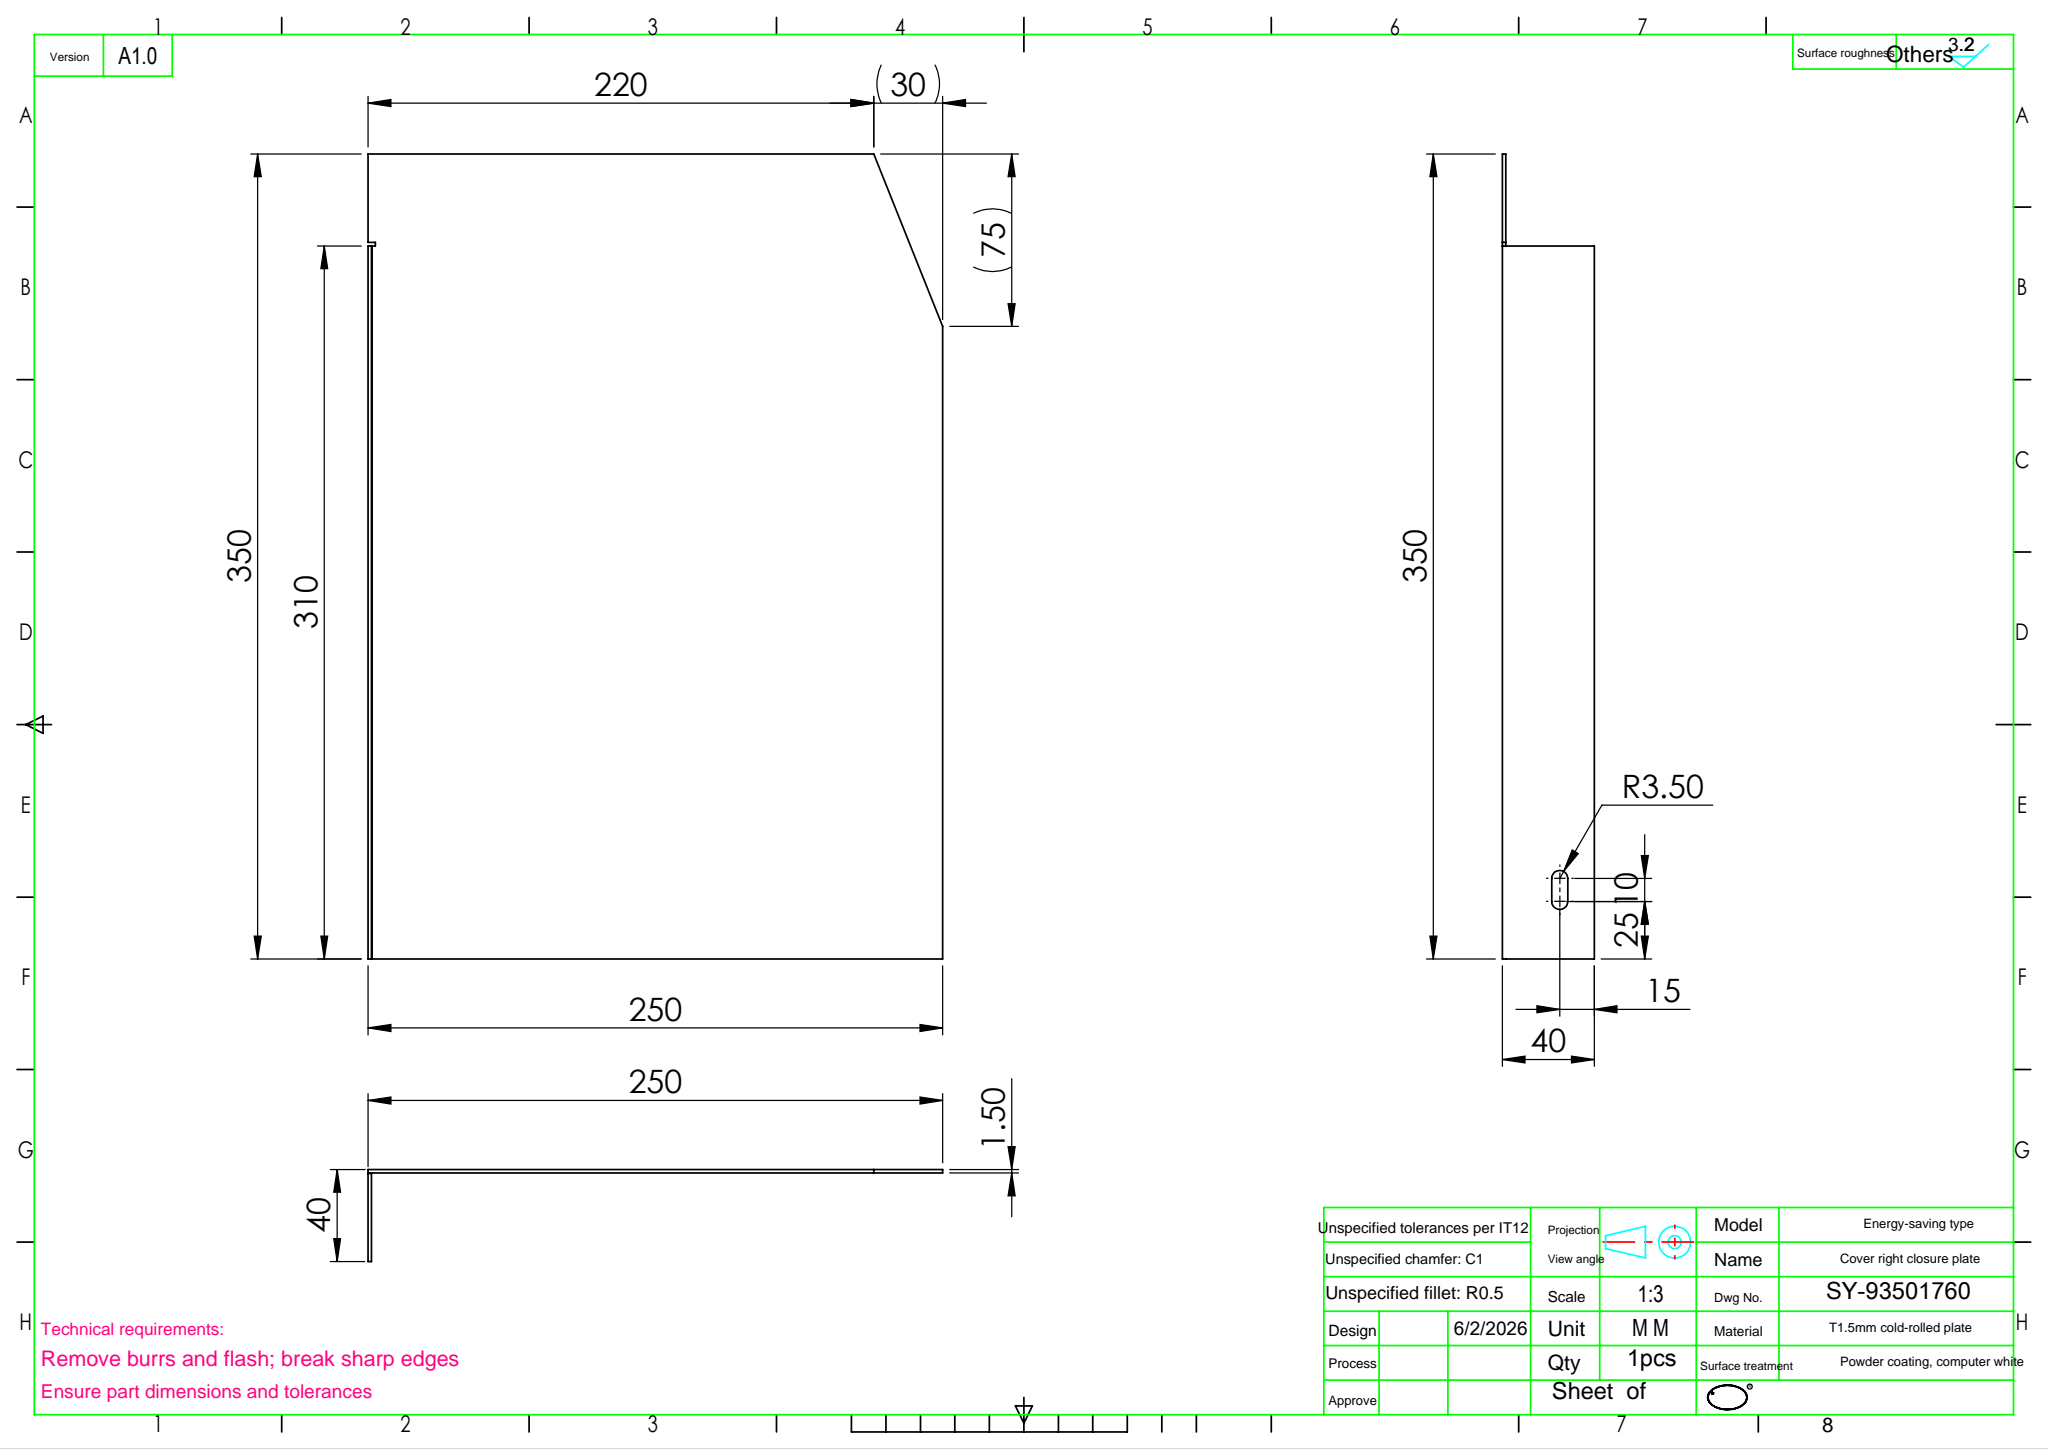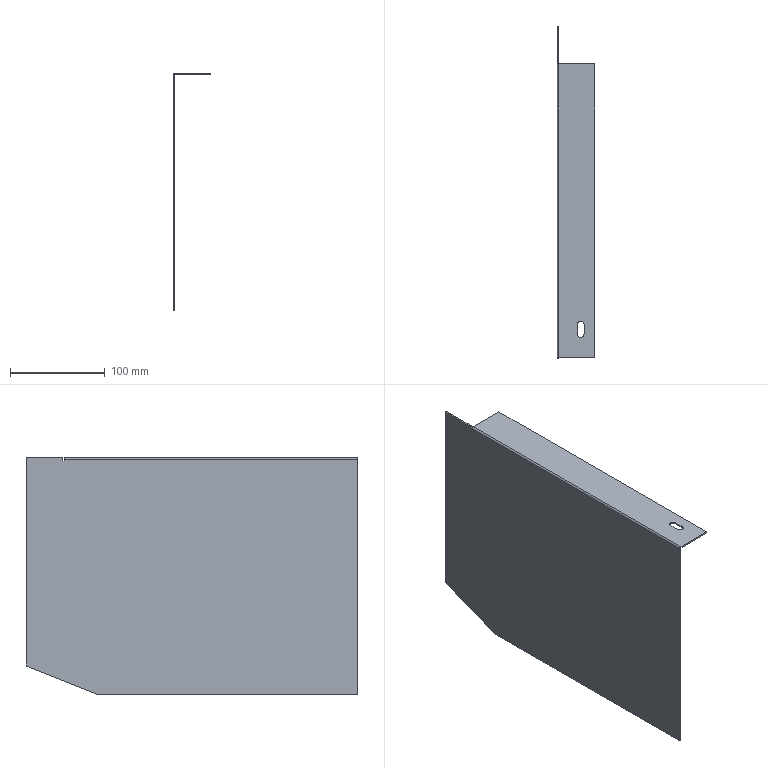Part | SolidWorks | features EdgeFlange 1, FlatPattern 1, ICE 1, SMBaseFlange 1, SheetMetal 1 | 1 solid | 24 faces | box 40 x 350 x 250 mm | volume 147105 mm3 | plane 19 | cylinder 5 | commonest cylinder face diameters 7 x3 0.4 x1 3.4 x1
STEP:
#1=CARTESIAN_POINT('',(23.5,38.5,0.));
#2=VERTEX_POINT('',#1);
#3=CARTESIAN_POINT('',(27.,35.,0.));
#4=VERTEX_POINT('',#3);
#5=CARTESIAN_POINT('',(23.5,35.,0.));
#6=DIRECTION('',(0.,0.,-1.));
#7=DIRECTION('',(-1.,0.,0.));
#8=AXIS2_PLACEMENT_3D('',#5,#6,#7);
#9=CIRCLE('',#8,3.5);
#10=EDGE_CURVE('',#2,#4,#9,.T.);
#11=ORIENTED_EDGE('',*,*,#10,.F.);
#12=CARTESIAN_POINT('',(23.5,38.5,-1.5));
#13=VERTEX_POINT('',#12);
#14=CARTESIAN_POINT('',(23.5,38.5,8.5));
#15=DIRECTION('',(0.,0.,-1.));
#16=VECTOR('',#15,1000.);
#17=LINE('',#14,#16);
#18=EDGE_CURVE('',#2,#13,#17,.T.);
#19=ORIENTED_EDGE('',*,*,#18,.T.);
#20=CARTESIAN_POINT('',(27.,35.,-1.5));
#21=VERTEX_POINT('',#20);
#22=CARTESIAN_POINT('',(23.5,35.,-1.5));
#23=DIRECTION('',(0.,0.,-1.));
#24=DIRECTION('',(0.,1.,0.));
#25=AXIS2_PLACEMENT_3D('',#22,#23,#24);
#26=CIRCLE('',#25,3.5);
#27=EDGE_CURVE('',#13,#21,#26,.T.);
#28=ORIENTED_EDGE('',*,*,#27,.T.);
#29=CARTESIAN_POINT('',(27.,35.,8.5));
#30=DIRECTION('',(0.,0.,-1.));
#31=VECTOR('',#30,1000.);
#32=LINE('',#29,#31);
#33=EDGE_CURVE('',#4,#21,#32,.T.);
#34=ORIENTED_EDGE('',*,*,#33,.F.);
#35=EDGE_LOOP('',(#11,#19,#28,#34));
#36=FACE_OUTER_BOUND('',#35,.T.);
#37=CARTESIAN_POINT('',(23.5,35.,8.5));
#38=DIRECTION('',(0.,0.,-1.));
#39=DIRECTION('',(0.,1.,0.));
#40=AXIS2_PLACEMENT_3D('',#37,#38,#39);
#41=CYLINDRICAL_SURFACE('',#40,3.5);
#42=ADVANCED_FACE('',(#36),#41,.F.);
#43=CARTESIAN_POINT('',(-1.5,350.,0.));
#44=VERTEX_POINT('',#43);
#45=CARTESIAN_POINT('',(-1.5,311.5,0.));
#46=VERTEX_POINT('',#45);
#47=CARTESIAN_POINT('',(-1.5,350.,0.));
#48=DIRECTION('',(0.,-1.,0.));
#49=VECTOR('',#48,1000.);
#50=LINE('',#47,#49);
#51=EDGE_CURVE('',#44,#46,#50,.T.);
#52=ORIENTED_EDGE('',*,*,#51,.T.);
#53=CARTESIAN_POINT('',(0.,311.5,0.));
#54=VERTEX_POINT('',#53);
#55=CARTESIAN_POINT('',(0.,311.5,0.));
#56=DIRECTION('',(-1.,0.,0.));
#57=VECTOR('',#56,1000.);
#58=LINE('',#55,#57);
#59=EDGE_CURVE('',#54,#46,#58,.T.);
#60=ORIENTED_EDGE('',*,*,#59,.F.);
#61=CARTESIAN_POINT('',(0.,350.,0.));
#62=VERTEX_POINT('',#61);
#63=CARTESIAN_POINT('',(0.,350.,0.));
#64=DIRECTION('',(0.,-1.,0.));
#65=VECTOR('',#64,1000.);
#66=LINE('',#63,#65);
#67=EDGE_CURVE('',#62,#54,#66,.T.);
#68=ORIENTED_EDGE('',*,*,#67,.F.);
#69=CARTESIAN_POINT('',(-1.5,350.,0.));
#70=DIRECTION('',(1.,0.,0.));
#71=VECTOR('',#70,1000.);
#72=LINE('',#69,#71);
#73=EDGE_CURVE('',#44,#62,#72,.T.);
#74=ORIENTED_EDGE('',*,*,#73,.F.);
#75=EDGE_LOOP('',(#52,#60,#68,#74));
#76=FACE_OUTER_BOUND('',#75,.T.);
#77=CARTESIAN_POINT('',(-1.5,350.,0.));
#78=DIRECTION('',(0.,0.,1.));
#79=DIRECTION('',(0.,-1.,0.));
#80=AXIS2_PLACEMENT_3D('',#77,#78,#79);
#81=PLANE('',#80);
#82=ADVANCED_FACE('',(#76),#81,.T.);
#83=CARTESIAN_POINT('',(0.,0.,-1.7));
#84=VERTEX_POINT('',#83);
#85=CARTESIAN_POINT('',(0.,0.,-250.));
#86=VERTEX_POINT('',#85);
#87=CARTESIAN_POINT('',(0.,0.,0.));
#88=DIRECTION('',(0.,0.,-1.));
#89=VECTOR('',#88,1000.);
#90=LINE('',#87,#89);
#91=EDGE_CURVE('',#84,#86,#90,.T.);
#92=ORIENTED_EDGE('',*,*,#91,.F.);
#93=CARTESIAN_POINT('',(-1.5,0.,-1.7));
#94=VERTEX_POINT('',#93);
#95=CARTESIAN_POINT('',(0.,0.,-1.7));
#96=DIRECTION('',(-1.,0.,0.));
#97=VECTOR('',#96,1000.);
#98=LINE('',#95,#97);
#99=EDGE_CURVE('',#84,#94,#98,.T.);
#100=ORIENTED_EDGE('',*,*,#99,.T.);
#101=CARTESIAN_POINT('',(-1.5,0.,-250.));
#102=VERTEX_POINT('',#101);
#103=CARTESIAN_POINT('',(-1.5,0.,0.));
#104=DIRECTION('',(0.,0.,-1.));
#105=VECTOR('',#104,1000.);
#106=LINE('',#103,#105);
#107=EDGE_CURVE('',#94,#102,#106,.T.);
#108=ORIENTED_EDGE('',*,*,#107,.T.);
#109=CARTESIAN_POINT('',(-1.5,0.,-250.));
#110=DIRECTION('',(1.,0.,0.));
#111=VECTOR('',#110,1000.);
#112=LINE('',#109,#111);
#113=EDGE_CURVE('',#102,#86,#112,.T.);
#114=ORIENTED_EDGE('',*,*,#113,.T.);
#115=EDGE_LOOP('',(#92,#100,#108,#114));
#116=FACE_OUTER_BOUND('',#115,.T.);
#117=CARTESIAN_POINT('',(-1.5,0.,0.));
#118=DIRECTION('',(0.,-1.,0.));
#119=DIRECTION('',(0.,0.,-1.));
#120=AXIS2_PLACEMENT_3D('',#117,#118,#119);
#121=PLANE('',#120);
#122=ADVANCED_FACE('',(#116),#121,.T.);
#123=CARTESIAN_POINT('',(-1.5,310.,-1.7));
#124=VERTEX_POINT('',#123);
#125=CARTESIAN_POINT('',(-1.5,0.,-1.7));
#126=DIRECTION('',(0.,1.,0.));
#127=VECTOR('',#126,1000.);
#128=LINE('',#125,#127);
#129=EDGE_CURVE('',#94,#124,#128,.T.);
#130=ORIENTED_EDGE('',*,*,#129,.T.);
#131=CARTESIAN_POINT('',(-1.5,310.,-3.2));
#132=VERTEX_POINT('',#131);
#133=CARTESIAN_POINT('',(-1.5,310.,0.));
#134=DIRECTION('',(0.,0.,1.));
#135=VECTOR('',#134,1000.);
#136=LINE('',#133,#135);
#137=EDGE_CURVE('',#132,#124,#136,.T.);
#138=ORIENTED_EDGE('',*,*,#137,.F.);
#139=CARTESIAN_POINT('',(-1.5,311.5,-3.2));
#140=VERTEX_POINT('',#139);
#141=CARTESIAN_POINT('',(-1.5,0.,-3.2));
#142=DIRECTION('',(0.,-1.,0.));
#143=VECTOR('',#142,1000.);
#144=LINE('',#141,#143);
#145=EDGE_CURVE('',#140,#132,#144,.T.);
#146=ORIENTED_EDGE('',*,*,#145,.F.);
#147=CARTESIAN_POINT('',(-1.5,311.5,0.));
#148=DIRECTION('',(0.,0.,-1.));
#149=VECTOR('',#148,1000.);
#150=LINE('',#147,#149);
#151=EDGE_CURVE('',#46,#140,#150,.T.);
#152=ORIENTED_EDGE('',*,*,#151,.F.);
#153=ORIENTED_EDGE('',*,*,#51,.F.);
#154=CARTESIAN_POINT('',(-1.5,350.,-220.));
#155=VERTEX_POINT('',#154);
#156=CARTESIAN_POINT('',(-1.5,350.,0.));
#157=DIRECTION('',(0.,0.,1.));
#158=VECTOR('',#157,1000.);
#159=LINE('',#156,#158);
#160=EDGE_CURVE('',#155,#44,#159,.T.);
#161=ORIENTED_EDGE('',*,*,#160,.F.);
#162=CARTESIAN_POINT('',(-1.5,275.,-250.));
#163=VERTEX_POINT('',#162);
#164=CARTESIAN_POINT('',(-1.5,350.,-220.));
#165=DIRECTION('',(0.,0.9285,0.3714));
#166=VECTOR('',#165,1000.);
#167=LINE('',#164,#166);
#168=EDGE_CURVE('',#163,#155,#167,.T.);
#169=ORIENTED_EDGE('',*,*,#168,.F.);
#170=CARTESIAN_POINT('',(-1.5,275.,-250.));
#171=DIRECTION('',(0.,1.,0.));
#172=VECTOR('',#171,1000.);
#173=LINE('',#170,#172);
#174=EDGE_CURVE('',#102,#163,#173,.T.);
#175=ORIENTED_EDGE('',*,*,#174,.F.);
#176=ORIENTED_EDGE('',*,*,#107,.F.);
#177=EDGE_LOOP('',(#130,#138,#146,#152,#153,#161,#169,#175,#176));
#178=FACE_OUTER_BOUND('',#177,.T.);
#179=CARTESIAN_POINT('',(-1.5,0.,0.));
#180=DIRECTION('',(1.,0.,0.));
#181=DIRECTION('',(0.,0.,-1.));
#182=AXIS2_PLACEMENT_3D('',#179,#180,#181);
#183=PLANE('',#182);
#184=ADVANCED_FACE('',(#178),#183,.F.);
#185=CARTESIAN_POINT('',(0.,310.,-1.7));
#186=VERTEX_POINT('',#185);
#187=CARTESIAN_POINT('',(0.,310.,-3.2));
#188=VERTEX_POINT('',#187);
#189=CARTESIAN_POINT('',(0.,310.,-1.7));
#190=DIRECTION('',(0.,0.,-1.));
#191=VECTOR('',#190,1000.);
#192=LINE('',#189,#191);
#193=EDGE_CURVE('',#186,#188,#192,.T.);
#194=ORIENTED_EDGE('',*,*,#193,.F.);
#195=CARTESIAN_POINT('',(0.,0.,-1.7));
#196=DIRECTION('',(0.,1.,0.));
#197=VECTOR('',#196,1000.);
#198=LINE('',#195,#197);
#199=EDGE_CURVE('',#84,#186,#198,.T.);
#200=ORIENTED_EDGE('',*,*,#199,.F.);
#201=ORIENTED_EDGE('',*,*,#91,.T.);
#202=CARTESIAN_POINT('',(0.,275.,-250.));
#203=VERTEX_POINT('',#202);
#204=CARTESIAN_POINT('',(0.,275.,-250.));
#205=DIRECTION('',(0.,1.,0.));
#206=VECTOR('',#205,1000.);
#207=LINE('',#204,#206);
#208=EDGE_CURVE('',#86,#203,#207,.T.);
#209=ORIENTED_EDGE('',*,*,#208,.T.);
#210=CARTESIAN_POINT('',(0.,350.,-220.));
#211=VERTEX_POINT('',#210);
#212=CARTESIAN_POINT('',(0.,350.,-220.));
#213=DIRECTION('',(0.,0.9285,0.3714));
#214=VECTOR('',#213,1000.);
#215=LINE('',#212,#214);
#216=EDGE_CURVE('',#203,#211,#215,.T.);
#217=ORIENTED_EDGE('',*,*,#216,.T.);
#218=CARTESIAN_POINT('',(0.,350.,0.));
#219=DIRECTION('',(0.,0.,1.));
#220=VECTOR('',#219,1000.);
#221=LINE('',#218,#220);
#222=EDGE_CURVE('',#211,#62,#221,.T.);
#223=ORIENTED_EDGE('',*,*,#222,.T.);
#224=ORIENTED_EDGE('',*,*,#67,.T.);
#225=CARTESIAN_POINT('',(0.,311.5,-3.2));
#226=VERTEX_POINT('',#225);
#227=CARTESIAN_POINT('',(0.,311.5,-3.2));
#228=DIRECTION('',(0.,0.,1.));
#229=VECTOR('',#228,1000.);
#230=LINE('',#227,#229);
#231=EDGE_CURVE('',#226,#54,#230,.T.);
#232=ORIENTED_EDGE('',*,*,#231,.F.);
#233=CARTESIAN_POINT('',(0.,310.,-3.2));
#234=DIRECTION('',(0.,1.,0.));
#235=VECTOR('',#234,1000.);
#236=LINE('',#233,#235);
#237=EDGE_CURVE('',#188,#226,#236,.T.);
#238=ORIENTED_EDGE('',*,*,#237,.F.);
#239=EDGE_LOOP('',(#194,#200,#201,#209,#217,#223,#224,#232,#238));
#240=FACE_OUTER_BOUND('',#239,.T.);
#241=CARTESIAN_POINT('',(0.,0.,0.));
#242=DIRECTION('',(1.,0.,0.));
#243=DIRECTION('',(0.,0.,-1.));
#244=AXIS2_PLACEMENT_3D('',#241,#242,#243);
#245=PLANE('',#244);
#246=ADVANCED_FACE('',(#240),#245,.T.);
#247=ORIENTED_EDGE('',*,*,#222,.F.);
#248=CARTESIAN_POINT('',(-1.5,350.,-220.));
#249=DIRECTION('',(1.,0.,0.));
#250=VECTOR('',#249,1000.);
#251=LINE('',#248,#250);
#252=EDGE_CURVE('',#155,#211,#251,.T.);
#253=ORIENTED_EDGE('',*,*,#252,.F.);
#254=ORIENTED_EDGE('',*,*,#160,.T.);
#255=ORIENTED_EDGE('',*,*,#73,.T.);
#256=EDGE_LOOP('',(#247,#253,#254,#255));
#257=FACE_OUTER_BOUND('',#256,.T.);
#258=CARTESIAN_POINT('',(-1.5,350.,0.));
#259=DIRECTION('',(0.,1.,0.));
#260=DIRECTION('',(0.,0.,1.));
#261=AXIS2_PLACEMENT_3D('',#258,#259,#260);
#262=PLANE('',#261);
#263=ADVANCED_FACE('',(#257),#262,.T.);
#264=ORIENTED_EDGE('',*,*,#216,.F.);
#265=CARTESIAN_POINT('',(-1.5,275.,-250.));
#266=DIRECTION('',(1.,0.,0.));
#267=VECTOR('',#266,1000.);
#268=LINE('',#265,#267);
#269=EDGE_CURVE('',#163,#203,#268,.T.);
#270=ORIENTED_EDGE('',*,*,#269,.F.);
#271=ORIENTED_EDGE('',*,*,#168,.T.);
#272=ORIENTED_EDGE('',*,*,#252,.T.);
#273=EDGE_LOOP('',(#264,#270,#271,#272));
#274=FACE_OUTER_BOUND('',#273,.T.);
#275=CARTESIAN_POINT('',(-1.5,350.,-220.));
#276=DIRECTION('',(0.,0.3714,-0.9285));
#277=DIRECTION('',(0.,0.9285,0.3714));
#278=AXIS2_PLACEMENT_3D('',#275,#276,#277);
#279=PLANE('',#278);
#280=ADVANCED_FACE('',(#274),#279,.T.);
#281=ORIENTED_EDGE('',*,*,#208,.F.);
#282=ORIENTED_EDGE('',*,*,#113,.F.);
#283=ORIENTED_EDGE('',*,*,#174,.T.);
#284=ORIENTED_EDGE('',*,*,#269,.T.);
#285=EDGE_LOOP('',(#281,#282,#283,#284));
#286=FACE_OUTER_BOUND('',#285,.T.);
#287=CARTESIAN_POINT('',(-1.5,275.,-250.));
#288=DIRECTION('',(0.,0.,-1.));
#289=DIRECTION('',(0.,1.,0.));
#290=AXIS2_PLACEMENT_3D('',#287,#288,#289);
#291=PLANE('',#290);
#292=ADVANCED_FACE('',(#286),#291,.T.);
#293=CARTESIAN_POINT('',(0.,310.,-3.2));
#294=DIRECTION('',(-1.,0.,0.));
#295=VECTOR('',#294,1000.);
#296=LINE('',#293,#295);
#297=EDGE_CURVE('',#188,#132,#296,.T.);
#298=ORIENTED_EDGE('',*,*,#297,.T.);
#299=ORIENTED_EDGE('',*,*,#137,.T.);
#300=CARTESIAN_POINT('',(0.,310.,-1.7));
#301=DIRECTION('',(-1.,0.,0.));
#302=VECTOR('',#301,1000.);
#303=LINE('',#300,#302);
#304=EDGE_CURVE('',#186,#124,#303,.T.);
#305=ORIENTED_EDGE('',*,*,#304,.F.);
#306=ORIENTED_EDGE('',*,*,#193,.T.);
#307=EDGE_LOOP('',(#298,#299,#305,#306));
#308=FACE_OUTER_BOUND('',#307,.T.);
#309=CARTESIAN_POINT('',(0.,310.,-1.7));
#310=DIRECTION('',(0.,1.,0.));
#311=DIRECTION('',(0.,0.,1.));
#312=AXIS2_PLACEMENT_3D('',#309,#310,#311);
#313=PLANE('',#312);
#314=ADVANCED_FACE('',(#308),#313,.T.);
#315=CARTESIAN_POINT('',(0.,311.5,-3.2));
#316=DIRECTION('',(-1.,0.,0.));
#317=VECTOR('',#316,1000.);
#318=LINE('',#315,#317);
#319=EDGE_CURVE('',#226,#140,#318,.T.);
#320=ORIENTED_EDGE('',*,*,#319,.T.);
#321=ORIENTED_EDGE('',*,*,#145,.T.);
#322=ORIENTED_EDGE('',*,*,#297,.F.);
#323=ORIENTED_EDGE('',*,*,#237,.T.);
#324=EDGE_LOOP('',(#320,#321,#322,#323));
#325=FACE_OUTER_BOUND('',#324,.T.);
#326=CARTESIAN_POINT('',(0.,310.,-3.2));
#327=DIRECTION('',(0.,0.,1.));
#328=DIRECTION('',(1.,0.,0.));
#329=AXIS2_PLACEMENT_3D('',#326,#327,#328);
#330=PLANE('',#329);
#331=ADVANCED_FACE('',(#325),#330,.T.);
#332=ORIENTED_EDGE('',*,*,#59,.T.);
#333=ORIENTED_EDGE('',*,*,#151,.T.);
#334=ORIENTED_EDGE('',*,*,#319,.F.);
#335=ORIENTED_EDGE('',*,*,#231,.T.);
#336=EDGE_LOOP('',(#332,#333,#334,#335));
#337=FACE_OUTER_BOUND('',#336,.T.);
#338=CARTESIAN_POINT('',(0.,311.5,-3.2));
#339=DIRECTION('',(0.,-1.,0.));
#340=DIRECTION('',(0.,0.,-1.));
#341=AXIS2_PLACEMENT_3D('',#338,#339,#340);
#342=PLANE('',#341);
#343=ADVANCED_FACE('',(#337),#342,.T.);
#344=CARTESIAN_POINT('',(0.2,310.,-1.5));
#345=VERTEX_POINT('',#344);
#346=CARTESIAN_POINT('',(0.2,310.,0.));
#347=VERTEX_POINT('',#346);
#348=CARTESIAN_POINT('',(0.2,310.,0.));
#349=DIRECTION('',(0.,0.,1.));
#350=VECTOR('',#349,1000.);
#351=LINE('',#348,#350);
#352=EDGE_CURVE('',#345,#347,#351,.T.);
#353=ORIENTED_EDGE('',*,*,#352,.F.);
#354=CARTESIAN_POINT('',(0.2,310.,-1.7));
#355=DIRECTION('',(0.,1.,0.));
#356=DIRECTION('',(0.,0.,-1.));
#357=AXIS2_PLACEMENT_3D('',#354,#355,#356);
#358=CIRCLE('',#357,0.2);
#359=EDGE_CURVE('',#186,#345,#358,.T.);
#360=ORIENTED_EDGE('',*,*,#359,.F.);
#361=ORIENTED_EDGE('',*,*,#304,.T.);
#362=CARTESIAN_POINT('',(0.2,310.,-1.7));
#363=DIRECTION('',(0.,1.,0.));
#364=DIRECTION('',(0.,0.,-1.));
#365=AXIS2_PLACEMENT_3D('',#362,#363,#364);
#366=CIRCLE('',#365,1.7);
#367=EDGE_CURVE('',#124,#347,#366,.T.);
#368=ORIENTED_EDGE('',*,*,#367,.T.);
#369=EDGE_LOOP('',(#353,#360,#361,#368));
#370=FACE_OUTER_BOUND('',#369,.T.);
#371=CARTESIAN_POINT('',(0.2,310.,-1.7));
#372=DIRECTION('',(0.,1.,0.));
#373=DIRECTION('',(0.,0.,1.));
#374=AXIS2_PLACEMENT_3D('',#371,#372,#373);
#375=PLANE('',#374);
#376=ADVANCED_FACE('',(#370),#375,.T.);
#377=CARTESIAN_POINT('',(0.2,0.,-1.5));
#378=VERTEX_POINT('',#377);
#379=CARTESIAN_POINT('',(0.2,0.,-1.7));
#380=DIRECTION('',(0.,-1.,0.));
#381=DIRECTION('',(0.,0.,-1.));
#382=AXIS2_PLACEMENT_3D('',#379,#380,#381);
#383=CIRCLE('',#382,0.2);
#384=EDGE_CURVE('',#378,#84,#383,.T.);
#385=ORIENTED_EDGE('',*,*,#384,.F.);
#386=CARTESIAN_POINT('',(0.2,0.,0.));
#387=VERTEX_POINT('',#386);
#388=CARTESIAN_POINT('',(0.2,0.,-1.5));
#389=DIRECTION('',(0.,0.,1.));
#390=VECTOR('',#389,1000.);
#391=LINE('',#388,#390);
#392=EDGE_CURVE('',#378,#387,#391,.T.);
#393=ORIENTED_EDGE('',*,*,#392,.T.);
#394=CARTESIAN_POINT('',(0.2,0.,-1.7));
#395=DIRECTION('',(0.,-1.,0.));
#396=DIRECTION('',(0.,0.,-1.));
#397=AXIS2_PLACEMENT_3D('',#394,#395,#396);
#398=CIRCLE('',#397,1.7);
#399=EDGE_CURVE('',#387,#94,#398,.T.);
#400=ORIENTED_EDGE('',*,*,#399,.T.);
#401=ORIENTED_EDGE('',*,*,#99,.F.);
#402=EDGE_LOOP('',(#385,#393,#400,#401));
#403=FACE_OUTER_BOUND('',#402,.T.);
#404=CARTESIAN_POINT('',(0.2,0.,-1.7));
#405=DIRECTION('',(0.,1.,0.));
#406=DIRECTION('',(0.,0.,1.));
#407=AXIS2_PLACEMENT_3D('',#404,#405,#406);
#408=PLANE('',#407);
#409=ADVANCED_FACE('',(#403),#408,.F.);
#410=ORIENTED_EDGE('',*,*,#129,.F.);
#411=ORIENTED_EDGE('',*,*,#399,.F.);
#412=CARTESIAN_POINT('',(0.2,310.,0.));
#413=DIRECTION('',(0.,1.,0.));
#414=VECTOR('',#413,1000.);
#415=LINE('',#412,#414);
#416=EDGE_CURVE('',#387,#347,#415,.T.);
#417=ORIENTED_EDGE('',*,*,#416,.T.);
#418=ORIENTED_EDGE('',*,*,#367,.F.);
#419=EDGE_LOOP('',(#410,#411,#417,#418));
#420=FACE_OUTER_BOUND('',#419,.T.);
#421=CARTESIAN_POINT('',(0.2,0.,-1.7));
#422=DIRECTION('',(0.,-1.,0.));
#423=DIRECTION('',(0.,0.,1.));
#424=AXIS2_PLACEMENT_3D('',#421,#422,#423);
#425=CYLINDRICAL_SURFACE('',#424,1.7);
#426=ADVANCED_FACE('',(#420),#425,.T.);
#427=ORIENTED_EDGE('',*,*,#199,.T.);
#428=ORIENTED_EDGE('',*,*,#359,.T.);
#429=CARTESIAN_POINT('',(0.2,310.,-1.5));
#430=DIRECTION('',(0.,-1.,0.));
#431=VECTOR('',#430,1000.);
#432=LINE('',#429,#431);
#433=EDGE_CURVE('',#345,#378,#432,.T.);
#434=ORIENTED_EDGE('',*,*,#433,.T.);
#435=ORIENTED_EDGE('',*,*,#384,.T.);
#436=EDGE_LOOP('',(#427,#428,#434,#435));
#437=FACE_OUTER_BOUND('',#436,.T.);
#438=CARTESIAN_POINT('',(0.2,0.,-1.7));
#439=DIRECTION('',(0.,-1.,0.));
#440=DIRECTION('',(0.,0.,1.));
#441=AXIS2_PLACEMENT_3D('',#438,#439,#440);
#442=CYLINDRICAL_SURFACE('',#441,0.2);
#443=ADVANCED_FACE('',(#437),#442,.F.);
#444=ORIENTED_EDGE('',*,*,#392,.F.);
#445=CARTESIAN_POINT('',(38.5,0.,-1.5));
#446=VERTEX_POINT('',#445);
#447=CARTESIAN_POINT('',(38.5,0.,-1.5));
#448=DIRECTION('',(1.,0.,0.));
#449=VECTOR('',#448,1000.);
#450=LINE('',#447,#449);
#451=EDGE_CURVE('',#378,#446,#450,.T.);
#452=ORIENTED_EDGE('',*,*,#451,.T.);
#453=CARTESIAN_POINT('',(38.5,0.,0.));
#454=VERTEX_POINT('',#453);
#455=CARTESIAN_POINT('',(38.5,0.,0.));
#456=DIRECTION('',(0.,0.,-1.));
#457=VECTOR('',#456,1000.);
#458=LINE('',#455,#457);
#459=EDGE_CURVE('',#454,#446,#458,.T.);
#460=ORIENTED_EDGE('',*,*,#459,.F.);
#461=CARTESIAN_POINT('',(0.,0.,0.));
#462=DIRECTION('',(1.,0.,0.));
#463=VECTOR('',#462,1000.);
#464=LINE('',#461,#463);
#465=EDGE_CURVE('',#387,#454,#464,.T.);
#466=ORIENTED_EDGE('',*,*,#465,.F.);
#467=EDGE_LOOP('',(#444,#452,#460,#466));
#468=FACE_OUTER_BOUND('',#467,.T.);
#469=CARTESIAN_POINT('',(38.5,0.,0.));
#470=DIRECTION('',(0.,1.,0.));
#471=DIRECTION('',(0.,0.,1.));
#472=AXIS2_PLACEMENT_3D('',#469,#470,#471);
#473=PLANE('',#472);
#474=ADVANCED_FACE('',(#468),#473,.F.);
#475=ORIENTED_EDGE('',*,*,#352,.T.);
#476=CARTESIAN_POINT('',(38.5,310.,0.));
#477=VERTEX_POINT('',#476);
#478=CARTESIAN_POINT('',(0.,310.,0.));
#479=DIRECTION('',(-1.,0.,0.));
#480=VECTOR('',#479,1000.);
#481=LINE('',#478,#480);
#482=EDGE_CURVE('',#477,#347,#481,.T.);
#483=ORIENTED_EDGE('',*,*,#482,.F.);
#484=CARTESIAN_POINT('',(38.5,310.,-1.5));
#485=VERTEX_POINT('',#484);
#486=CARTESIAN_POINT('',(38.5,310.,0.));
#487=DIRECTION('',(0.,0.,-1.));
#488=VECTOR('',#487,1000.);
#489=LINE('',#486,#488);
#490=EDGE_CURVE('',#477,#485,#489,.T.);
#491=ORIENTED_EDGE('',*,*,#490,.T.);
#492=CARTESIAN_POINT('',(0.,310.,-1.5));
#493=DIRECTION('',(-1.,0.,0.));
#494=VECTOR('',#493,1000.);
#495=LINE('',#492,#494);
#496=EDGE_CURVE('',#485,#345,#495,.T.);
#497=ORIENTED_EDGE('',*,*,#496,.T.);
#498=EDGE_LOOP('',(#475,#483,#491,#497));
#499=FACE_OUTER_BOUND('',#498,.T.);
#500=CARTESIAN_POINT('',(0.,310.,0.));
#501=DIRECTION('',(0.,-1.,0.));
#502=DIRECTION('',(0.,0.,-1.));
#503=AXIS2_PLACEMENT_3D('',#500,#501,#502);
#504=PLANE('',#503);
#505=ADVANCED_FACE('',(#499),#504,.F.);
#506=CARTESIAN_POINT('',(20.,25.,0.));
#507=VERTEX_POINT('',#506);
#508=CARTESIAN_POINT('',(20.,35.,0.));
#509=VERTEX_POINT('',#508);
#510=CARTESIAN_POINT('',(20.,0.,0.));
#511=DIRECTION('',(0.,1.,0.));
#512=VECTOR('',#511,1000.);
#513=LINE('',#510,#512);
#514=EDGE_CURVE('',#507,#509,#513,.T.);
#515=ORIENTED_EDGE('',*,*,#514,.T.);
#516=CARTESIAN_POINT('',(23.5,35.,0.));
#517=DIRECTION('',(0.,0.,-1.));
#518=DIRECTION('',(-1.,0.,0.));
#519=AXIS2_PLACEMENT_3D('',#516,#517,#518);
#520=CIRCLE('',#519,3.5);
#521=EDGE_CURVE('',#509,#2,#520,.T.);
#522=ORIENTED_EDGE('',*,*,#521,.T.);
#523=ORIENTED_EDGE('',*,*,#10,.T.);
#524=CARTESIAN_POINT('',(27.,25.,0.));
#525=VERTEX_POINT('',#524);
#526=CARTESIAN_POINT('',(27.,0.,0.));
#527=DIRECTION('',(0.,-1.,0.));
#528=VECTOR('',#527,1000.);
#529=LINE('',#526,#528);
#530=EDGE_CURVE('',#4,#525,#529,.T.);
#531=ORIENTED_EDGE('',*,*,#530,.T.);
#532=CARTESIAN_POINT('',(23.5,25.,0.));
#533=DIRECTION('',(0.,0.,-1.));
#534=DIRECTION('',(-1.,0.,0.));
#535=AXIS2_PLACEMENT_3D('',#532,#533,#534);
#536=CIRCLE('',#535,3.5);
#537=EDGE_CURVE('',#525,#507,#536,.T.);
#538=ORIENTED_EDGE('',*,*,#537,.T.);
#539=EDGE_LOOP('',(#515,#522,#523,#531,#538));
#540=FACE_BOUND('',#539,.T.);
#541=ORIENTED_EDGE('',*,*,#416,.F.);
#542=ORIENTED_EDGE('',*,*,#465,.T.);
#543=CARTESIAN_POINT('',(38.5,0.,0.));
#544=DIRECTION('',(0.,1.,0.));
#545=VECTOR('',#544,1000.);
#546=LINE('',#543,#545);
#547=EDGE_CURVE('',#454,#477,#546,.T.);
#548=ORIENTED_EDGE('',*,*,#547,.T.);
#549=ORIENTED_EDGE('',*,*,#482,.T.);
#550=EDGE_LOOP('',(#541,#542,#548,#549));
#551=FACE_OUTER_BOUND('',#550,.T.);
#552=CARTESIAN_POINT('',(0.,0.,0.));
#553=DIRECTION('',(0.,0.,-1.));
#554=DIRECTION('',(-1.,0.,0.));
#555=AXIS2_PLACEMENT_3D('',#552,#553,#554);
#556=PLANE('',#555);
#557=ADVANCED_FACE('',(#540,#551),#556,.F.);
#558=CARTESIAN_POINT('',(20.,35.,-1.5));
#559=VERTEX_POINT('',#558);
#560=CARTESIAN_POINT('',(23.5,35.,-1.5));
#561=DIRECTION('',(0.,0.,-1.));
#562=DIRECTION('',(0.,1.,0.));
#563=AXIS2_PLACEMENT_3D('',#560,#561,#562);
#564=CIRCLE('',#563,3.5);
#565=EDGE_CURVE('',#559,#13,#564,.T.);
#566=ORIENTED_EDGE('',*,*,#565,.F.);
#567=CARTESIAN_POINT('',(20.,25.,-1.5));
#568=VERTEX_POINT('',#567);
#569=CARTESIAN_POINT('',(20.,35.,-1.5));
#570=DIRECTION('',(0.,1.,0.));
#571=VECTOR('',#570,1000.);
#572=LINE('',#569,#571);
#573=EDGE_CURVE('',#568,#559,#572,.T.);
#574=ORIENTED_EDGE('',*,*,#573,.F.);
#575=CARTESIAN_POINT('',(27.,25.,-1.5));
#576=VERTEX_POINT('',#575);
#577=CARTESIAN_POINT('',(23.5,25.,-1.5));
#578=DIRECTION('',(0.,0.,-1.));
#579=DIRECTION('',(0.,1.,0.));
#580=AXIS2_PLACEMENT_3D('',#577,#578,#579);
#581=CIRCLE('',#580,3.5);
#582=EDGE_CURVE('',#576,#568,#581,.T.);
#583=ORIENTED_EDGE('',*,*,#582,.F.);
#584=CARTESIAN_POINT('',(27.,35.,-1.5));
#585=DIRECTION('',(0.,-1.,0.));
#586=VECTOR('',#585,1000.);
#587=LINE('',#584,#586);
#588=EDGE_CURVE('',#21,#576,#587,.T.);
#589=ORIENTED_EDGE('',*,*,#588,.F.);
#590=ORIENTED_EDGE('',*,*,#27,.F.);
#591=EDGE_LOOP('',(#566,#574,#583,#589,#590));
#592=FACE_BOUND('',#591,.T.);
#593=ORIENTED_EDGE('',*,*,#451,.F.);
#594=ORIENTED_EDGE('',*,*,#433,.F.);
#595=ORIENTED_EDGE('',*,*,#496,.F.);
#596=CARTESIAN_POINT('',(38.5,310.,-1.5));
#597=DIRECTION('',(0.,1.,0.));
#598=VECTOR('',#597,1000.);
#599=LINE('',#596,#598);
#600=EDGE_CURVE('',#446,#485,#599,.T.);
#601=ORIENTED_EDGE('',*,*,#600,.F.);
#602=EDGE_LOOP('',(#593,#594,#595,#601));
#603=FACE_OUTER_BOUND('',#602,.T.);
#604=CARTESIAN_POINT('',(0.,0.,-1.5));
#605=DIRECTION('',(0.,0.,-1.));
#606=DIRECTION('',(-1.,0.,0.));
#607=AXIS2_PLACEMENT_3D('',#604,#605,#606);
#608=PLANE('',#607);
#609=ADVANCED_FACE('',(#592,#603),#608,.T.);
#610=ORIENTED_EDGE('',*,*,#600,.T.);
#611=ORIENTED_EDGE('',*,*,#490,.F.);
#612=ORIENTED_EDGE('',*,*,#547,.F.);
#613=ORIENTED_EDGE('',*,*,#459,.T.);
#614=EDGE_LOOP('',(#610,#611,#612,#613));
#615=FACE_OUTER_BOUND('',#614,.T.);
#616=CARTESIAN_POINT('',(38.5,310.,0.));
#617=DIRECTION('',(-1.,0.,0.));
#618=DIRECTION('',(0.,0.,1.));
#619=AXIS2_PLACEMENT_3D('',#616,#617,#618);
#620=PLANE('',#619);
#621=ADVANCED_FACE('',(#615),#620,.F.);
#622=ORIENTED_EDGE('',*,*,#18,.F.);
#623=ORIENTED_EDGE('',*,*,#521,.F.);
#624=CARTESIAN_POINT('',(20.,35.,8.5));
#625=DIRECTION('',(0.,0.,-1.));
#626=VECTOR('',#625,1000.);
#627=LINE('',#624,#626);
#628=EDGE_CURVE('',#509,#559,#627,.T.);
#629=ORIENTED_EDGE('',*,*,#628,.T.);
#630=ORIENTED_EDGE('',*,*,#565,.T.);
#631=EDGE_LOOP('',(#622,#623,#629,#630));
#632=FACE_OUTER_BOUND('',#631,.T.);
#633=CARTESIAN_POINT('',(23.5,35.,8.5));
#634=DIRECTION('',(0.,0.,-1.));
#635=DIRECTION('',(0.,1.,0.));
#636=AXIS2_PLACEMENT_3D('',#633,#634,#635);
#637=CYLINDRICAL_SURFACE('',#636,3.5);
#638=ADVANCED_FACE('',(#632),#637,.F.);
#639=CARTESIAN_POINT('',(20.,25.,8.5));
#640=DIRECTION('',(0.,0.,-1.));
#641=VECTOR('',#640,1000.);
#642=LINE('',#639,#641);
#643=EDGE_CURVE('',#507,#568,#642,.T.);
#644=ORIENTED_EDGE('',*,*,#643,.T.);
#645=ORIENTED_EDGE('',*,*,#573,.T.);
#646=ORIENTED_EDGE('',*,*,#628,.F.);
#647=ORIENTED_EDGE('',*,*,#514,.F.);
#648=EDGE_LOOP('',(#644,#645,#646,#647));
#649=FACE_OUTER_BOUND('',#648,.T.);
#650=CARTESIAN_POINT('',(20.,35.,8.5));
#651=DIRECTION('',(-1.,0.,0.));
#652=DIRECTION('',(0.,-1.,0.));
#653=AXIS2_PLACEMENT_3D('',#650,#651,#652);
#654=PLANE('',#653);
#655=ADVANCED_FACE('',(#649),#654,.F.);
#656=CARTESIAN_POINT('',(27.,25.,8.5));
#657=DIRECTION('',(0.,0.,-1.));
#658=VECTOR('',#657,1000.);
#659=LINE('',#656,#658);
#660=EDGE_CURVE('',#525,#576,#659,.T.);
#661=ORIENTED_EDGE('',*,*,#660,.T.);
#662=ORIENTED_EDGE('',*,*,#582,.T.);
#663=ORIENTED_EDGE('',*,*,#643,.F.);
#664=ORIENTED_EDGE('',*,*,#537,.F.);
#665=EDGE_LOOP('',(#661,#662,#663,#664));
#666=FACE_OUTER_BOUND('',#665,.T.);
#667=CARTESIAN_POINT('',(23.5,25.,8.5));
#668=DIRECTION('',(0.,0.,-1.));
#669=DIRECTION('',(0.,1.,0.));
#670=AXIS2_PLACEMENT_3D('',#667,#668,#669);
#671=CYLINDRICAL_SURFACE('',#670,3.5);
#672=ADVANCED_FACE('',(#666),#671,.F.);
#673=ORIENTED_EDGE('',*,*,#33,.T.);
#674=ORIENTED_EDGE('',*,*,#588,.T.);
#675=ORIENTED_EDGE('',*,*,#660,.F.);
#676=ORIENTED_EDGE('',*,*,#530,.F.);
#677=EDGE_LOOP('',(#673,#674,#675,#676));
#678=FACE_OUTER_BOUND('',#677,.T.);
#679=CARTESIAN_POINT('',(27.,35.,8.5));
#680=DIRECTION('',(1.,0.,0.));
#681=DIRECTION('',(0.,1.,0.));
#682=AXIS2_PLACEMENT_3D('',#679,#680,#681);
#683=PLANE('',#682);
#684=ADVANCED_FACE('',(#678),#683,.F.);
#685=CLOSED_SHELL('',(#42,#82,#122,#184,#246,#263,#280,#292,#314,#331,#343,#376,#409,#426,#443,#474,#505,#557,#609,#621,#638,#655,#672,#684));
#686=MANIFOLD_SOLID_BREP('',#685);
#687=CARTESIAN_POINT('',(0.,0.,0.));
#688=DIRECTION('',(0.,0.,1.));
#689=DIRECTION('',(1.,0.,0.));
#690=AXIS2_PLACEMENT_3D('',#687,#688,#689);
#691=(LENGTH_UNIT()NAMED_UNIT(*)SI_UNIT(.MILLI.,.METRE.));
#692=UNCERTAINTY_MEASURE_WITH_UNIT(LENGTH_MEASURE(0.00001),#691,'','');
#693=(NAMED_UNIT(*)PLANE_ANGLE_UNIT()SI_UNIT($,.RADIAN.));
#694=(NAMED_UNIT(*)SI_UNIT($,.STERADIAN.)SOLID_ANGLE_UNIT());
#695=(GEOMETRIC_REPRESENTATION_CONTEXT(3)GLOBAL_UNCERTAINTY_ASSIGNED_CONTEXT((#692))GLOBAL_UNIT_ASSIGNED_CONTEXT((#691,#693,#694))REPRESENTATION_CONTEXT('',''));
#696=ADVANCED_BREP_SHAPE_REPRESENTATION('',(#686,#690),#695);